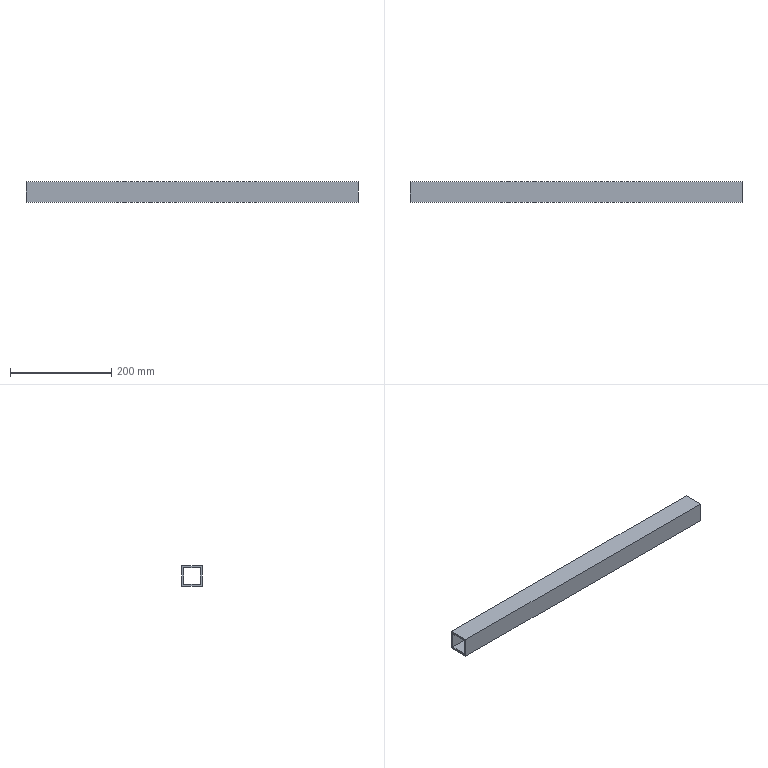Part | NX | features solid 2 | 1 solid | 10 faces | box 655 x 40 x 40 mm | volume 377280 mm3 | plane 10
STEP:
#1=CARTESIAN_POINT('',(485.,-20.,-45.));
#2=VERTEX_POINT('',#1);
#3=CARTESIAN_POINT('',(485.,-20.,-85.));
#4=VERTEX_POINT('',#3);
#5=CARTESIAN_POINT('',(485.,-20.,-40.));
#6=DIRECTION('',(0.,0.,-1.));
#7=VECTOR('',#6,1000.);
#8=LINE('',#5,#7);
#9=EDGE_CURVE('',#2,#4,#8,.T.);
#10=ORIENTED_EDGE('',*,*,#9,.F.);
#11=CARTESIAN_POINT('',(1140.,-20.,-45.));
#12=VERTEX_POINT('',#11);
#13=CARTESIAN_POINT('',(204.393,-20.,-45.));
#14=DIRECTION('',(-1.,0.,0.));
#15=VECTOR('',#14,1000.);
#16=LINE('',#13,#15);
#17=EDGE_CURVE('',#12,#2,#16,.T.);
#18=ORIENTED_EDGE('',*,*,#17,.F.);
#19=CARTESIAN_POINT('',(1140.,-20.,-85.));
#20=VERTEX_POINT('',#19);
#21=CARTESIAN_POINT('',(1140.,-20.,-40.));
#22=DIRECTION('',(0.,0.,1.));
#23=VECTOR('',#22,1000.);
#24=LINE('',#21,#23);
#25=EDGE_CURVE('',#20,#12,#24,.T.);
#26=ORIENTED_EDGE('',*,*,#25,.F.);
#27=CARTESIAN_POINT('',(204.393,-20.,-85.));
#28=DIRECTION('',(1.,0.,0.));
#29=VECTOR('',#28,1000.);
#30=LINE('',#27,#29);
#31=EDGE_CURVE('',#4,#20,#30,.T.);
#32=ORIENTED_EDGE('',*,*,#31,.F.);
#33=EDGE_LOOP('',(#10,#18,#26,#32));
#34=FACE_BOUND('',#33,.T.);
#35=CARTESIAN_POINT('',(119.393,-20.,-40.));
#36=DIRECTION('',(0.,-1.,0.));
#37=DIRECTION('',(0.,0.,-1.));
#38=AXIS2_PLACEMENT_3D('',#35,#36,#37);
#39=PLANE('',#38);
#40=ADVANCED_FACE('',(#34),#39,.F.);
#41=CARTESIAN_POINT('',(485.,-60.,-45.));
#42=VERTEX_POINT('',#41);
#43=CARTESIAN_POINT('',(485.,-680.,-45.));
#44=DIRECTION('',(0.,1.,0.));
#45=VECTOR('',#44,1000.);
#46=LINE('',#43,#45);
#47=EDGE_CURVE('',#42,#2,#46,.T.);
#48=ORIENTED_EDGE('',*,*,#47,.F.);
#49=CARTESIAN_POINT('',(1140.,-60.,-45.));
#50=VERTEX_POINT('',#49);
#51=CARTESIAN_POINT('',(204.393,-60.,-45.));
#52=DIRECTION('',(1.,0.,0.));
#53=VECTOR('',#52,1000.);
#54=LINE('',#51,#53);
#55=EDGE_CURVE('',#42,#50,#54,.T.);
#56=ORIENTED_EDGE('',*,*,#55,.T.);
#57=CARTESIAN_POINT('',(1140.,-680.,-45.));
#58=DIRECTION('',(0.,-1.,0.));
#59=VECTOR('',#58,1000.);
#60=LINE('',#57,#59);
#61=EDGE_CURVE('',#12,#50,#60,.T.);
#62=ORIENTED_EDGE('',*,*,#61,.F.);
#63=ORIENTED_EDGE('',*,*,#17,.T.);
#64=EDGE_LOOP('',(#48,#56,#62,#63));
#65=FACE_BOUND('',#64,.T.);
#66=CARTESIAN_POINT('',(204.393,-680.,-45.));
#67=DIRECTION('',(0.,0.,-1.));
#68=DIRECTION('',(0.,1.,0.));
#69=AXIS2_PLACEMENT_3D('',#66,#67,#68);
#70=PLANE('',#69);
#71=ADVANCED_FACE('',(#65),#70,.F.);
#72=CARTESIAN_POINT('',(485.,-60.,-85.));
#73=VERTEX_POINT('',#72);
#74=CARTESIAN_POINT('',(485.,-640.,-85.));
#75=DIRECTION('',(0.,-1.,0.));
#76=VECTOR('',#75,1000.);
#77=LINE('',#74,#76);
#78=EDGE_CURVE('',#4,#73,#77,.T.);
#79=ORIENTED_EDGE('',*,*,#78,.F.);
#80=ORIENTED_EDGE('',*,*,#31,.T.);
#81=CARTESIAN_POINT('',(1140.,-60.,-85.));
#82=VERTEX_POINT('',#81);
#83=CARTESIAN_POINT('',(1140.,-640.,-85.));
#84=DIRECTION('',(0.,1.,0.));
#85=VECTOR('',#84,1000.);
#86=LINE('',#83,#85);
#87=EDGE_CURVE('',#82,#20,#86,.T.);
#88=ORIENTED_EDGE('',*,*,#87,.F.);
#89=CARTESIAN_POINT('',(119.393,-60.,-85.));
#90=DIRECTION('',(1.,0.,0.));
#91=VECTOR('',#90,1000.);
#92=LINE('',#89,#91);
#93=EDGE_CURVE('',#73,#82,#92,.T.);
#94=ORIENTED_EDGE('',*,*,#93,.F.);
#95=EDGE_LOOP('',(#79,#80,#88,#94));
#96=FACE_BOUND('',#95,.T.);
#97=CARTESIAN_POINT('',(204.393,-640.,-85.));
#98=DIRECTION('',(0.,0.,1.));
#99=DIRECTION('',(0.,-1.,0.));
#100=AXIS2_PLACEMENT_3D('',#97,#98,#99);
#101=PLANE('',#100);
#102=ADVANCED_FACE('',(#96),#101,.F.);
#103=CARTESIAN_POINT('',(485.,-60.,-70.));
#104=DIRECTION('',(0.,0.,1.));
#105=VECTOR('',#104,1000.);
#106=LINE('',#103,#105);
#107=EDGE_CURVE('',#73,#42,#106,.T.);
#108=ORIENTED_EDGE('',*,*,#107,.F.);
#109=ORIENTED_EDGE('',*,*,#93,.T.);
#110=CARTESIAN_POINT('',(1140.,-60.,-70.));
#111=DIRECTION('',(0.,0.,-1.));
#112=VECTOR('',#111,1000.);
#113=LINE('',#110,#112);
#114=EDGE_CURVE('',#50,#82,#113,.T.);
#115=ORIENTED_EDGE('',*,*,#114,.F.);
#116=ORIENTED_EDGE('',*,*,#55,.F.);
#117=EDGE_LOOP('',(#108,#109,#115,#116));
#118=FACE_BOUND('',#117,.T.);
#119=CARTESIAN_POINT('',(119.393,-60.,-70.));
#120=DIRECTION('',(0.,1.,0.));
#121=DIRECTION('',(0.,0.,1.));
#122=AXIS2_PLACEMENT_3D('',#119,#120,#121);
#123=PLANE('',#122);
#124=ADVANCED_FACE('',(#118),#123,.F.);
#125=CARTESIAN_POINT('',(1140.,-56.,-49.));
#126=VERTEX_POINT('',#125);
#127=CARTESIAN_POINT('',(1140.,-56.,-81.));
#128=VERTEX_POINT('',#127);
#129=CARTESIAN_POINT('',(1140.,-56.,-70.));
#130=DIRECTION('',(0.,0.,-1.));
#131=VECTOR('',#130,1000.);
#132=LINE('',#129,#131);
#133=EDGE_CURVE('',#126,#128,#132,.T.);
#134=ORIENTED_EDGE('',*,*,#133,.F.);
#135=CARTESIAN_POINT('',(1140.,-24.,-49.));
#136=VERTEX_POINT('',#135);
#137=CARTESIAN_POINT('',(1140.,-680.,-49.));
#138=DIRECTION('',(0.,-1.,0.));
#139=VECTOR('',#138,1000.);
#140=LINE('',#137,#139);
#141=EDGE_CURVE('',#136,#126,#140,.T.);
#142=ORIENTED_EDGE('',*,*,#141,.F.);
#143=CARTESIAN_POINT('',(1140.,-24.,-81.));
#144=VERTEX_POINT('',#143);
#145=CARTESIAN_POINT('',(1140.,-24.,-40.));
#146=DIRECTION('',(0.,0.,1.));
#147=VECTOR('',#146,1000.);
#148=LINE('',#145,#147);
#149=EDGE_CURVE('',#144,#136,#148,.T.);
#150=ORIENTED_EDGE('',*,*,#149,.F.);
#151=CARTESIAN_POINT('',(1140.,-640.,-81.));
#152=DIRECTION('',(0.,1.,0.));
#153=VECTOR('',#152,1000.);
#154=LINE('',#151,#153);
#155=EDGE_CURVE('',#128,#144,#154,.T.);
#156=ORIENTED_EDGE('',*,*,#155,.F.);
#157=EDGE_LOOP('',(#134,#142,#150,#156));
#158=FACE_BOUND('',#157,.T.);
#159=ORIENTED_EDGE('',*,*,#61,.T.);
#160=ORIENTED_EDGE('',*,*,#114,.T.);
#161=ORIENTED_EDGE('',*,*,#87,.T.);
#162=ORIENTED_EDGE('',*,*,#25,.T.);
#163=EDGE_LOOP('',(#159,#160,#161,#162));
#164=FACE_BOUND('',#163,.T.);
#165=CARTESIAN_POINT('',(1140.,-87.5,-9.5));
#166=DIRECTION('',(1.,0.,0.));
#167=DIRECTION('',(0.,0.,-1.));
#168=AXIS2_PLACEMENT_3D('',#165,#166,#167);
#169=PLANE('',#168);
#170=ADVANCED_FACE('',(#158,#164),#169,.T.);
#171=CARTESIAN_POINT('',(485.,-24.,-49.));
#172=VERTEX_POINT('',#171);
#173=CARTESIAN_POINT('',(204.393,-24.,-49.));
#174=DIRECTION('',(-1.,0.,0.));
#175=VECTOR('',#174,1000.);
#176=LINE('',#173,#175);
#177=EDGE_CURVE('',#136,#172,#176,.T.);
#178=ORIENTED_EDGE('',*,*,#177,.T.);
#179=CARTESIAN_POINT('',(485.,-24.,-81.));
#180=VERTEX_POINT('',#179);
#181=CARTESIAN_POINT('',(485.,-24.,-40.));
#182=DIRECTION('',(0.,0.,-1.));
#183=VECTOR('',#182,1000.);
#184=LINE('',#181,#183);
#185=EDGE_CURVE('',#172,#180,#184,.T.);
#186=ORIENTED_EDGE('',*,*,#185,.T.);
#187=CARTESIAN_POINT('',(204.393,-24.,-81.));
#188=DIRECTION('',(1.,0.,0.));
#189=VECTOR('',#188,1000.);
#190=LINE('',#187,#189);
#191=EDGE_CURVE('',#180,#144,#190,.T.);
#192=ORIENTED_EDGE('',*,*,#191,.T.);
#193=ORIENTED_EDGE('',*,*,#149,.T.);
#194=EDGE_LOOP('',(#178,#186,#192,#193));
#195=FACE_BOUND('',#194,.T.);
#196=CARTESIAN_POINT('',(119.393,-24.,-40.));
#197=DIRECTION('',(0.,-1.,0.));
#198=DIRECTION('',(0.,0.,-1.));
#199=AXIS2_PLACEMENT_3D('',#196,#197,#198);
#200=PLANE('',#199);
#201=ADVANCED_FACE('',(#195),#200,.T.);
#202=CARTESIAN_POINT('',(485.,-56.,-49.));
#203=VERTEX_POINT('',#202);
#204=CARTESIAN_POINT('',(204.393,-56.,-49.));
#205=DIRECTION('',(1.,0.,0.));
#206=VECTOR('',#205,1000.);
#207=LINE('',#204,#206);
#208=EDGE_CURVE('',#203,#126,#207,.T.);
#209=ORIENTED_EDGE('',*,*,#208,.F.);
#210=CARTESIAN_POINT('',(485.,-680.,-49.));
#211=DIRECTION('',(0.,1.,0.));
#212=VECTOR('',#211,1000.);
#213=LINE('',#210,#212);
#214=EDGE_CURVE('',#203,#172,#213,.T.);
#215=ORIENTED_EDGE('',*,*,#214,.T.);
#216=ORIENTED_EDGE('',*,*,#177,.F.);
#217=ORIENTED_EDGE('',*,*,#141,.T.);
#218=EDGE_LOOP('',(#209,#215,#216,#217));
#219=FACE_BOUND('',#218,.T.);
#220=CARTESIAN_POINT('',(204.393,-680.,-49.));
#221=DIRECTION('',(0.,0.,-1.));
#222=DIRECTION('',(0.,1.,0.));
#223=AXIS2_PLACEMENT_3D('',#220,#221,#222);
#224=PLANE('',#223);
#225=ADVANCED_FACE('',(#219),#224,.T.);
#226=ORIENTED_EDGE('',*,*,#191,.F.);
#227=CARTESIAN_POINT('',(485.,-56.,-81.));
#228=VERTEX_POINT('',#227);
#229=CARTESIAN_POINT('',(485.,-640.,-81.));
#230=DIRECTION('',(0.,-1.,0.));
#231=VECTOR('',#230,1000.);
#232=LINE('',#229,#231);
#233=EDGE_CURVE('',#180,#228,#232,.T.);
#234=ORIENTED_EDGE('',*,*,#233,.T.);
#235=CARTESIAN_POINT('',(119.393,-56.,-81.));
#236=DIRECTION('',(1.,0.,0.));
#237=VECTOR('',#236,1000.);
#238=LINE('',#235,#237);
#239=EDGE_CURVE('',#228,#128,#238,.T.);
#240=ORIENTED_EDGE('',*,*,#239,.T.);
#241=ORIENTED_EDGE('',*,*,#155,.T.);
#242=EDGE_LOOP('',(#226,#234,#240,#241));
#243=FACE_BOUND('',#242,.T.);
#244=CARTESIAN_POINT('',(204.393,-640.,-81.));
#245=DIRECTION('',(0.,0.,1.));
#246=DIRECTION('',(0.,-1.,0.));
#247=AXIS2_PLACEMENT_3D('',#244,#245,#246);
#248=PLANE('',#247);
#249=ADVANCED_FACE('',(#243),#248,.T.);
#250=ORIENTED_EDGE('',*,*,#239,.F.);
#251=CARTESIAN_POINT('',(485.,-56.,-70.));
#252=DIRECTION('',(0.,0.,1.));
#253=VECTOR('',#252,1000.);
#254=LINE('',#251,#253);
#255=EDGE_CURVE('',#228,#203,#254,.T.);
#256=ORIENTED_EDGE('',*,*,#255,.T.);
#257=ORIENTED_EDGE('',*,*,#208,.T.);
#258=ORIENTED_EDGE('',*,*,#133,.T.);
#259=EDGE_LOOP('',(#250,#256,#257,#258));
#260=FACE_BOUND('',#259,.T.);
#261=CARTESIAN_POINT('',(119.393,-56.,-70.));
#262=DIRECTION('',(0.,1.,0.));
#263=DIRECTION('',(0.,0.,1.));
#264=AXIS2_PLACEMENT_3D('',#261,#262,#263);
#265=PLANE('',#264);
#266=ADVANCED_FACE('',(#260),#265,.T.);
#267=ORIENTED_EDGE('',*,*,#255,.F.);
#268=ORIENTED_EDGE('',*,*,#233,.F.);
#269=ORIENTED_EDGE('',*,*,#185,.F.);
#270=ORIENTED_EDGE('',*,*,#214,.F.);
#271=EDGE_LOOP('',(#267,#268,#269,#270));
#272=FACE_BOUND('',#271,.T.);
#273=ORIENTED_EDGE('',*,*,#78,.T.);
#274=ORIENTED_EDGE('',*,*,#107,.T.);
#275=ORIENTED_EDGE('',*,*,#47,.T.);
#276=ORIENTED_EDGE('',*,*,#9,.T.);
#277=EDGE_LOOP('',(#273,#274,#275,#276));
#278=FACE_BOUND('',#277,.T.);
#279=CARTESIAN_POINT('',(485.,-30.4,2.));
#280=DIRECTION('',(-1.,0.,0.));
#281=DIRECTION('',(0.,0.,1.));
#282=AXIS2_PLACEMENT_3D('',#279,#280,#281);
#283=PLANE('',#282);
#284=ADVANCED_FACE('',(#272,#278),#283,.T.);
#285=CLOSED_SHELL('',(#40,#71,#102,#124,#170,#201,#225,#249,#266,#284));
#286=MANIFOLD_SOLID_BREP('',#285);
#287=(LENGTH_UNIT()NAMED_UNIT(*)SI_UNIT(.MILLI.,.METRE.));
#288=UNCERTAINTY_MEASURE_WITH_UNIT(LENGTH_MEASURE(0.00001),#287,'','');
#289=(NAMED_UNIT(*)PLANE_ANGLE_UNIT()SI_UNIT($,.RADIAN.));
#290=(NAMED_UNIT(*)SI_UNIT($,.STERADIAN.)SOLID_ANGLE_UNIT());
#291=(GEOMETRIC_REPRESENTATION_CONTEXT(3)GLOBAL_UNCERTAINTY_ASSIGNED_CONTEXT((#288))GLOBAL_UNIT_ASSIGNED_CONTEXT((#287,#289,#290))REPRESENTATION_CONTEXT('',''));
#292=ADVANCED_BREP_SHAPE_REPRESENTATION('',(#286),#291);